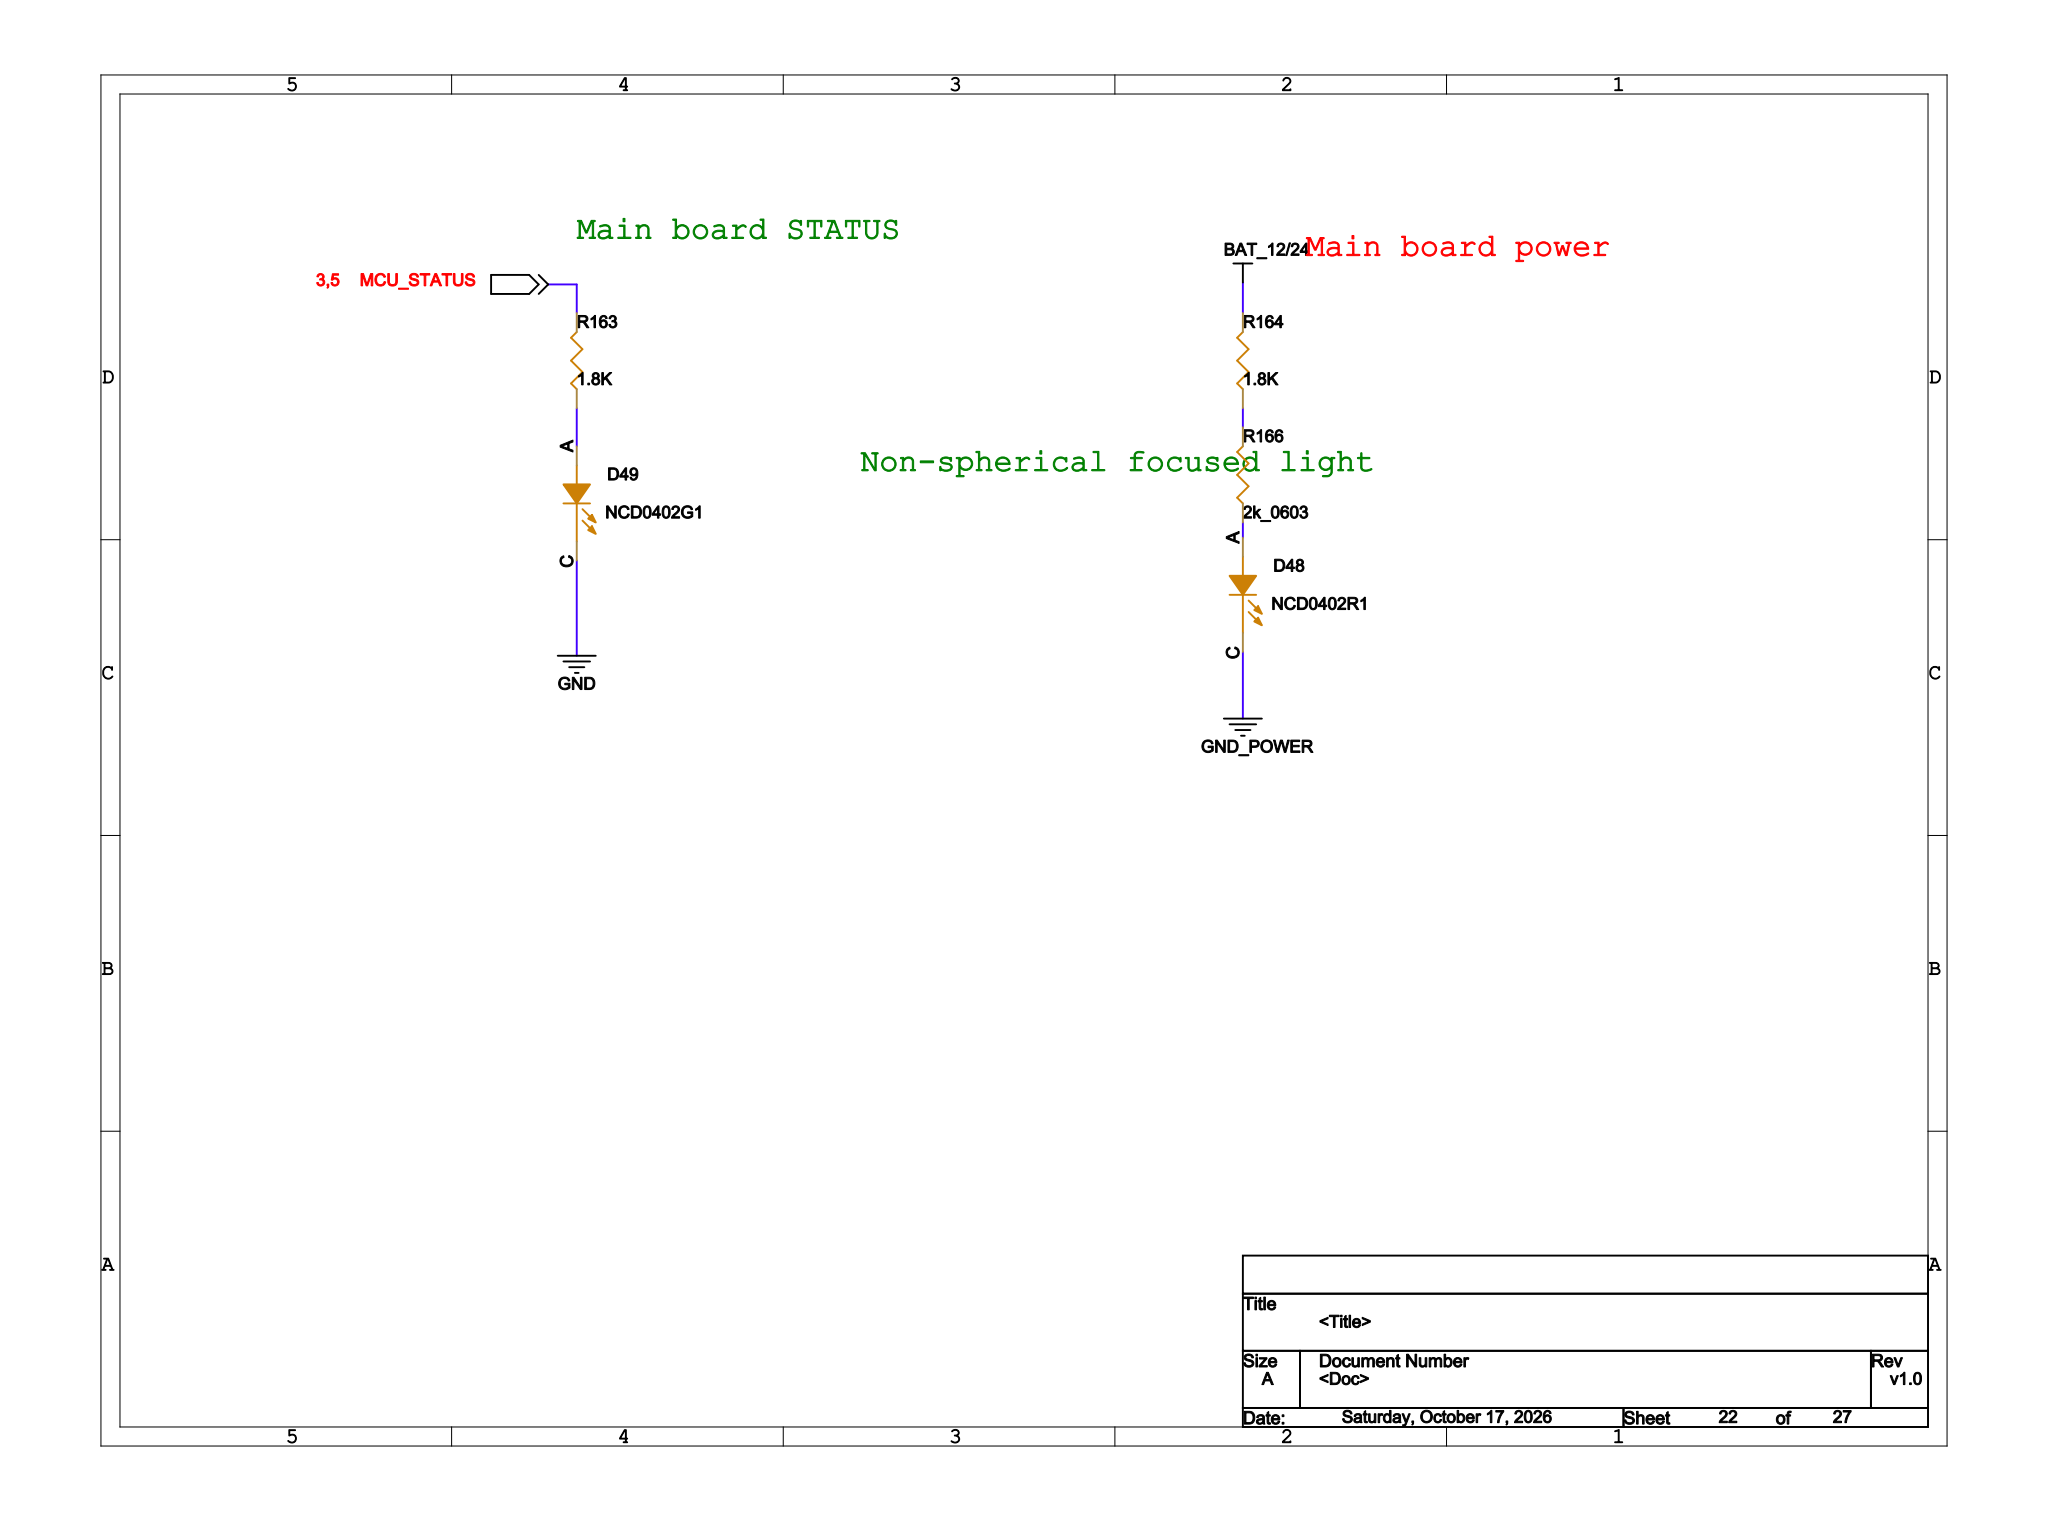Circuit board | Cadence Allegro | 477 parts | 327 nets | one sheet of the schematic
Parts on this sheet (reference | value | footprint):
D48 | NCD0402R1 | LED0402_H050
D49 | NCD0402G1 | LED0402_H050
R163 | 1.8K | 0402
R164 | 1.8K | 0402
R166 | 2k_0603 | 0603
Nets of these parts (net: part-pin ...):
GND: D49-C
BAT_GND: D48-C
N16934741: D48-A R166-1
N16781465: R164-1 R166-2
N16781463: D49-A R163-1
MCU_STATUS: R163-2
BAT_12/24: R164-2